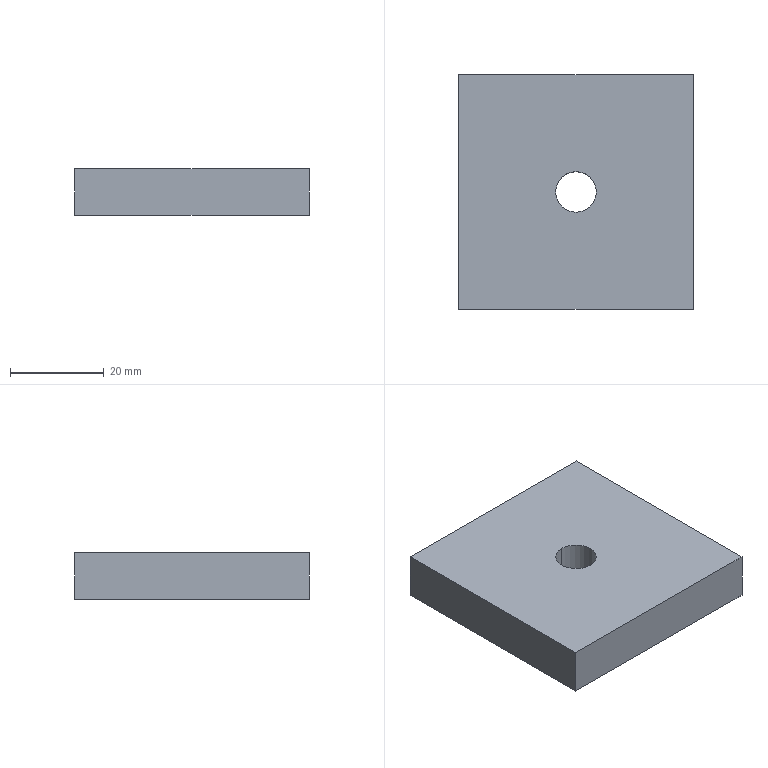Part | NX | features solid 2 | 1 solid | 8 faces | box 50 x 50 x 10 mm | volume 24413 mm3 | plane 6 | cylinder 2 | commonest cylinder face diameters 8.647 x2
STEP:
#1=CARTESIAN_POINT('',(-960.,20.677,1305.));
#2=VERTEX_POINT('',#1);
#3=CARTESIAN_POINT('',(-960.,20.677,1295.));
#4=VERTEX_POINT('',#3);
#5=CARTESIAN_POINT('',(-960.,20.677,1366.414));
#6=DIRECTION('',(0.,0.,-1.));
#7=VECTOR('',#6,1000.);
#8=LINE('',#5,#7);
#9=EDGE_CURVE('',#2,#4,#8,.T.);
#10=ORIENTED_EDGE('',*,*,#9,.F.);
#11=CARTESIAN_POINT('',(-960.,29.324,1305.));
#12=VERTEX_POINT('',#11);
#13=CARTESIAN_POINT('',(-960.,25.,1305.));
#14=DIRECTION('',(0.,0.,-1.));
#15=DIRECTION('',(0.,1.,0.));
#16=AXIS2_PLACEMENT_3D('',#13,#14,#15);
#17=CIRCLE('',#16,4.324);
#18=EDGE_CURVE('',#12,#2,#17,.T.);
#19=ORIENTED_EDGE('',*,*,#18,.F.);
#20=CARTESIAN_POINT('',(-960.,29.324,1295.));
#21=VERTEX_POINT('',#20);
#22=CARTESIAN_POINT('',(-960.,29.324,1366.414));
#23=DIRECTION('',(0.,0.,-1.));
#24=VECTOR('',#23,1000.);
#25=LINE('',#22,#24);
#26=EDGE_CURVE('',#21,#12,#25,.F.);
#27=ORIENTED_EDGE('',*,*,#26,.F.);
#28=CARTESIAN_POINT('',(-960.,25.,1295.));
#29=DIRECTION('',(0.,0.,-1.));
#30=DIRECTION('',(0.,1.,0.));
#31=AXIS2_PLACEMENT_3D('',#28,#29,#30);
#32=CIRCLE('',#31,4.324);
#33=EDGE_CURVE('',#21,#4,#32,.T.);
#34=ORIENTED_EDGE('',*,*,#33,.T.);
#35=EDGE_LOOP('',(#10,#19,#27,#34));
#36=FACE_BOUND('',#35,.T.);
#37=CARTESIAN_POINT('',(-960.,25.,1366.414));
#38=DIRECTION('',(0.,0.,-1.));
#39=DIRECTION('',(0.,1.,0.));
#40=AXIS2_PLACEMENT_3D('',#37,#38,#39);
#41=CYLINDRICAL_SURFACE('',#40,4.324);
#42=ADVANCED_FACE('',(#36),#41,.F.);
#43=ORIENTED_EDGE('',*,*,#18,.T.);
#44=CARTESIAN_POINT('',(-960.,25.,1305.));
#45=DIRECTION('',(0.,0.,-1.));
#46=DIRECTION('',(0.,1.,0.));
#47=AXIS2_PLACEMENT_3D('',#44,#45,#46);
#48=CIRCLE('',#47,4.324);
#49=EDGE_CURVE('',#2,#12,#48,.T.);
#50=ORIENTED_EDGE('',*,*,#49,.T.);
#51=EDGE_LOOP('',(#43,#50));
#52=FACE_BOUND('',#51,.T.);
#53=CARTESIAN_POINT('',(-935.,0.,1305.));
#54=VERTEX_POINT('',#53);
#55=CARTESIAN_POINT('',(-985.,0.,1305.));
#56=VERTEX_POINT('',#55);
#57=CARTESIAN_POINT('',(-935.,0.,1305.));
#58=DIRECTION('',(-1.,0.,0.));
#59=VECTOR('',#58,1000.);
#60=LINE('',#57,#59);
#61=EDGE_CURVE('',#54,#56,#60,.T.);
#62=ORIENTED_EDGE('',*,*,#61,.F.);
#63=CARTESIAN_POINT('',(-935.,50.,1305.));
#64=VERTEX_POINT('',#63);
#65=CARTESIAN_POINT('',(-935.,50.,1305.));
#66=DIRECTION('',(0.,-1.,0.));
#67=VECTOR('',#66,1000.);
#68=LINE('',#65,#67);
#69=EDGE_CURVE('',#64,#54,#68,.T.);
#70=ORIENTED_EDGE('',*,*,#69,.F.);
#71=CARTESIAN_POINT('',(-985.,50.,1305.));
#72=VERTEX_POINT('',#71);
#73=CARTESIAN_POINT('',(-985.,50.,1305.));
#74=DIRECTION('',(1.,0.,0.));
#75=VECTOR('',#74,1000.);
#76=LINE('',#73,#75);
#77=EDGE_CURVE('',#72,#64,#76,.T.);
#78=ORIENTED_EDGE('',*,*,#77,.F.);
#79=CARTESIAN_POINT('',(-985.,0.,1305.));
#80=DIRECTION('',(0.,1.,0.));
#81=VECTOR('',#80,1000.);
#82=LINE('',#79,#81);
#83=EDGE_CURVE('',#56,#72,#82,.T.);
#84=ORIENTED_EDGE('',*,*,#83,.F.);
#85=EDGE_LOOP('',(#62,#70,#78,#84));
#86=FACE_BOUND('',#85,.T.);
#87=CARTESIAN_POINT('',(-980.548,11.252,1305.));
#88=DIRECTION('',(0.,0.,-1.));
#89=DIRECTION('',(0.,-1.,0.));
#90=AXIS2_PLACEMENT_3D('',#87,#88,#89);
#91=PLANE('',#90);
#92=ADVANCED_FACE('',(#52,#86),#91,.F.);
#93=ORIENTED_EDGE('',*,*,#33,.F.);
#94=CARTESIAN_POINT('',(-960.,25.,1295.));
#95=DIRECTION('',(0.,0.,-1.));
#96=DIRECTION('',(0.,1.,0.));
#97=AXIS2_PLACEMENT_3D('',#94,#95,#96);
#98=CIRCLE('',#97,4.324);
#99=EDGE_CURVE('',#4,#21,#98,.T.);
#100=ORIENTED_EDGE('',*,*,#99,.F.);
#101=EDGE_LOOP('',(#93,#100));
#102=FACE_BOUND('',#101,.T.);
#103=CARTESIAN_POINT('',(-935.,0.,1295.));
#104=VERTEX_POINT('',#103);
#105=CARTESIAN_POINT('',(-985.,0.,1295.));
#106=VERTEX_POINT('',#105);
#107=CARTESIAN_POINT('',(-935.,0.,1295.));
#108=DIRECTION('',(-1.,0.,0.));
#109=VECTOR('',#108,1000.);
#110=LINE('',#107,#109);
#111=EDGE_CURVE('',#104,#106,#110,.T.);
#112=ORIENTED_EDGE('',*,*,#111,.T.);
#113=CARTESIAN_POINT('',(-985.,50.,1295.));
#114=VERTEX_POINT('',#113);
#115=CARTESIAN_POINT('',(-985.,0.,1295.));
#116=DIRECTION('',(0.,1.,0.));
#117=VECTOR('',#116,1000.);
#118=LINE('',#115,#117);
#119=EDGE_CURVE('',#106,#114,#118,.T.);
#120=ORIENTED_EDGE('',*,*,#119,.T.);
#121=CARTESIAN_POINT('',(-935.,50.,1295.));
#122=VERTEX_POINT('',#121);
#123=CARTESIAN_POINT('',(-985.,50.,1295.));
#124=DIRECTION('',(1.,0.,0.));
#125=VECTOR('',#124,1000.);
#126=LINE('',#123,#125);
#127=EDGE_CURVE('',#114,#122,#126,.T.);
#128=ORIENTED_EDGE('',*,*,#127,.T.);
#129=CARTESIAN_POINT('',(-935.,50.,1295.));
#130=DIRECTION('',(0.,-1.,0.));
#131=VECTOR('',#130,1000.);
#132=LINE('',#129,#131);
#133=EDGE_CURVE('',#122,#104,#132,.T.);
#134=ORIENTED_EDGE('',*,*,#133,.T.);
#135=EDGE_LOOP('',(#112,#120,#128,#134));
#136=FACE_BOUND('',#135,.T.);
#137=CARTESIAN_POINT('',(-980.548,11.252,1295.));
#138=DIRECTION('',(0.,0.,-1.));
#139=DIRECTION('',(0.,-1.,0.));
#140=AXIS2_PLACEMENT_3D('',#137,#138,#139);
#141=PLANE('',#140);
#142=ADVANCED_FACE('',(#102,#136),#141,.T.);
#143=ORIENTED_EDGE('',*,*,#69,.T.);
#144=CARTESIAN_POINT('',(-935.,0.,1295.));
#145=DIRECTION('',(0.,0.,1.));
#146=VECTOR('',#145,1000.);
#147=LINE('',#144,#146);
#148=EDGE_CURVE('',#104,#54,#147,.T.);
#149=ORIENTED_EDGE('',*,*,#148,.F.);
#150=ORIENTED_EDGE('',*,*,#133,.F.);
#151=CARTESIAN_POINT('',(-935.,50.,1295.));
#152=DIRECTION('',(0.,0.,1.));
#153=VECTOR('',#152,1000.);
#154=LINE('',#151,#153);
#155=EDGE_CURVE('',#122,#64,#154,.T.);
#156=ORIENTED_EDGE('',*,*,#155,.T.);
#157=EDGE_LOOP('',(#143,#149,#150,#156));
#158=FACE_BOUND('',#157,.T.);
#159=CARTESIAN_POINT('',(-935.,50.,1295.));
#160=DIRECTION('',(-1.,0.,0.));
#161=DIRECTION('',(0.,0.,1.));
#162=AXIS2_PLACEMENT_3D('',#159,#160,#161);
#163=PLANE('',#162);
#164=ADVANCED_FACE('',(#158),#163,.F.);
#165=ORIENTED_EDGE('',*,*,#77,.T.);
#166=ORIENTED_EDGE('',*,*,#155,.F.);
#167=ORIENTED_EDGE('',*,*,#127,.F.);
#168=CARTESIAN_POINT('',(-985.,50.,1295.));
#169=DIRECTION('',(0.,0.,1.));
#170=VECTOR('',#169,1000.);
#171=LINE('',#168,#170);
#172=EDGE_CURVE('',#114,#72,#171,.T.);
#173=ORIENTED_EDGE('',*,*,#172,.T.);
#174=EDGE_LOOP('',(#165,#166,#167,#173));
#175=FACE_BOUND('',#174,.T.);
#176=CARTESIAN_POINT('',(-985.,50.,1295.));
#177=DIRECTION('',(0.,-1.,0.));
#178=DIRECTION('',(-1.,0.,0.));
#179=AXIS2_PLACEMENT_3D('',#176,#177,#178);
#180=PLANE('',#179);
#181=ADVANCED_FACE('',(#175),#180,.F.);
#182=ORIENTED_EDGE('',*,*,#83,.T.);
#183=ORIENTED_EDGE('',*,*,#172,.F.);
#184=ORIENTED_EDGE('',*,*,#119,.F.);
#185=CARTESIAN_POINT('',(-985.,0.,1295.));
#186=DIRECTION('',(0.,0.,1.));
#187=VECTOR('',#186,1000.);
#188=LINE('',#185,#187);
#189=EDGE_CURVE('',#106,#56,#188,.T.);
#190=ORIENTED_EDGE('',*,*,#189,.T.);
#191=EDGE_LOOP('',(#182,#183,#184,#190));
#192=FACE_BOUND('',#191,.T.);
#193=CARTESIAN_POINT('',(-985.,0.,1295.));
#194=DIRECTION('',(1.,0.,0.));
#195=DIRECTION('',(0.,0.,1.));
#196=AXIS2_PLACEMENT_3D('',#193,#194,#195);
#197=PLANE('',#196);
#198=ADVANCED_FACE('',(#192),#197,.F.);
#199=ORIENTED_EDGE('',*,*,#61,.T.);
#200=ORIENTED_EDGE('',*,*,#189,.F.);
#201=ORIENTED_EDGE('',*,*,#111,.F.);
#202=ORIENTED_EDGE('',*,*,#148,.T.);
#203=EDGE_LOOP('',(#199,#200,#201,#202));
#204=FACE_BOUND('',#203,.T.);
#205=CARTESIAN_POINT('',(-935.,0.,1295.));
#206=DIRECTION('',(0.,1.,0.));
#207=DIRECTION('',(1.,0.,0.));
#208=AXIS2_PLACEMENT_3D('',#205,#206,#207);
#209=PLANE('',#208);
#210=ADVANCED_FACE('',(#204),#209,.F.);
#211=ORIENTED_EDGE('',*,*,#49,.F.);
#212=ORIENTED_EDGE('',*,*,#9,.T.);
#213=ORIENTED_EDGE('',*,*,#99,.T.);
#214=ORIENTED_EDGE('',*,*,#26,.T.);
#215=EDGE_LOOP('',(#211,#212,#213,#214));
#216=FACE_BOUND('',#215,.T.);
#217=CARTESIAN_POINT('',(-960.,25.,1366.414));
#218=DIRECTION('',(0.,0.,-1.));
#219=DIRECTION('',(0.,1.,0.));
#220=AXIS2_PLACEMENT_3D('',#217,#218,#219);
#221=CYLINDRICAL_SURFACE('',#220,4.324);
#222=ADVANCED_FACE('',(#216),#221,.F.);
#223=CLOSED_SHELL('',(#42,#92,#142,#164,#181,#198,#210,#222));
#224=MANIFOLD_SOLID_BREP('',#223);
#225=(LENGTH_UNIT()NAMED_UNIT(*)SI_UNIT(.MILLI.,.METRE.));
#226=UNCERTAINTY_MEASURE_WITH_UNIT(LENGTH_MEASURE(0.00001),#225,'','');
#227=(NAMED_UNIT(*)PLANE_ANGLE_UNIT()SI_UNIT($,.RADIAN.));
#228=(NAMED_UNIT(*)SI_UNIT($,.STERADIAN.)SOLID_ANGLE_UNIT());
#229=(GEOMETRIC_REPRESENTATION_CONTEXT(3)GLOBAL_UNCERTAINTY_ASSIGNED_CONTEXT((#226))GLOBAL_UNIT_ASSIGNED_CONTEXT((#225,#227,#228))REPRESENTATION_CONTEXT('',''));
#230=ADVANCED_BREP_SHAPE_REPRESENTATION('',(#224),#229);